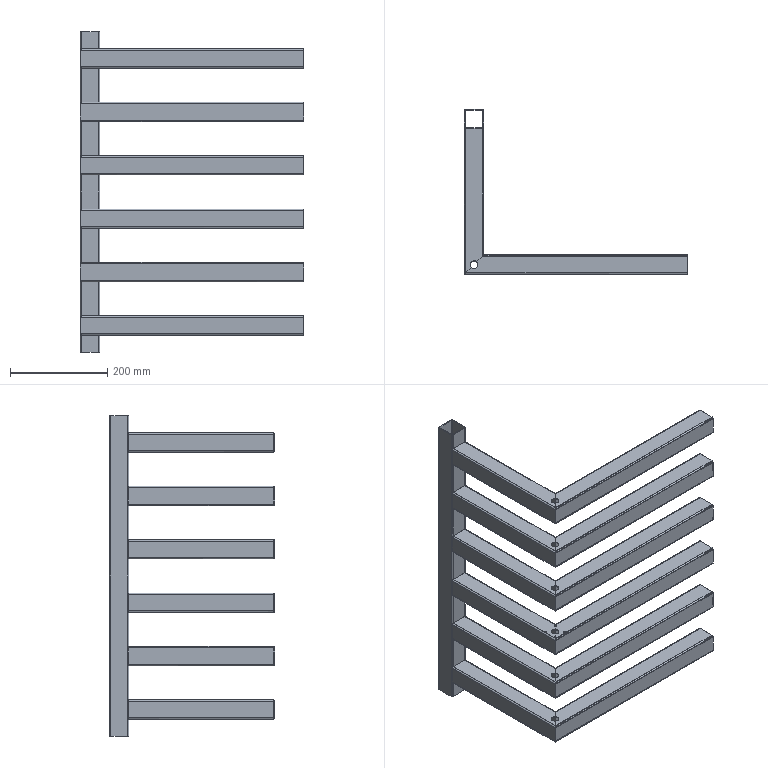Part | SolidWorks | features 3DProfileFeature 1, CirPattern 1, HoleWzd 1, ICE 1, LPattern 1, MirrorPattern 1, MirrorSolid 1, SMBaseFlange 1, WeldMemberFeat 1, WeldmentFeature 1 | 13 solids | 310 faces | box 460 x 340 x 660 mm | volume 1117739 mm3 | cylinder 160 | plane 150 | commonest cylinder face diameters 3 x52 6 x52 16 x36 4.2 x20